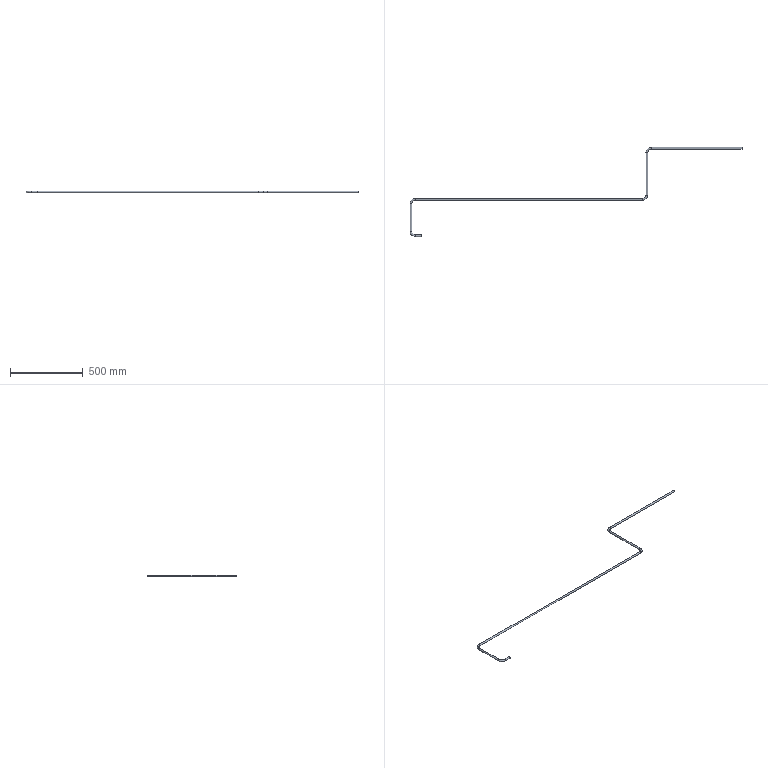Part | NX | features solid 2 | 1 solid | 11 faces | box 2287 x 613.706 x 12 mm | volume 328684 mm3 | cylinder 5 | torus 4 | plane 2 | commonest cylinder face diameters 12 x5
STEP:
#1=CARTESIAN_POINT('',(830.,756.706,-484.));
#2=VERTEX_POINT('',#1);
#3=CARTESIAN_POINT('',(830.,756.706,-490.));
#4=DIRECTION('',(1.,0.,0.));
#5=DIRECTION('',(0.,0.,1.));
#6=AXIS2_PLACEMENT_3D('',#3,#4,#5);
#7=CIRCLE('',#6,6.);
#8=EDGE_CURVE('',#2,#2,#7,.T.);
#9=ORIENTED_EDGE('',*,*,#8,.T.);
#10=EDGE_LOOP('',(#9));
#11=FACE_BOUND('',#10,.T.);
#12=CARTESIAN_POINT('',(1456.,756.706,-484.));
#13=VERTEX_POINT('',#12);
#14=CARTESIAN_POINT('',(1456.,756.706,-490.));
#15=DIRECTION('',(1.,0.,0.));
#16=DIRECTION('',(0.,0.,1.));
#17=AXIS2_PLACEMENT_3D('',#14,#15,#16);
#18=CIRCLE('',#17,6.);
#19=EDGE_CURVE('',#13,#13,#18,.T.);
#20=ORIENTED_EDGE('',*,*,#19,.F.);
#21=EDGE_LOOP('',(#20));
#22=FACE_BOUND('',#21,.T.);
#23=CARTESIAN_POINT('',(830.,756.706,-490.));
#24=DIRECTION('',(1.,0.,0.));
#25=DIRECTION('',(0.,1.,0.));
#26=AXIS2_PLACEMENT_3D('',#23,#24,#25);
#27=CYLINDRICAL_SURFACE('',#26,6.);
#28=ADVANCED_FACE('',(#11,#22),#27,.T.);
#29=CARTESIAN_POINT('',(800.,726.706,-484.));
#30=VERTEX_POINT('',#29);
#31=CARTESIAN_POINT('',(800.,726.706,-490.));
#32=DIRECTION('',(0.,1.,0.));
#33=DIRECTION('',(0.,0.,1.));
#34=AXIS2_PLACEMENT_3D('',#31,#32,#33);
#35=CIRCLE('',#34,6.);
#36=EDGE_CURVE('',#30,#30,#35,.T.);
#37=ORIENTED_EDGE('',*,*,#36,.T.);
#38=EDGE_LOOP('',(#37));
#39=FACE_BOUND('',#38,.T.);
#40=ORIENTED_EDGE('',*,*,#8,.F.);
#41=EDGE_LOOP('',(#40));
#42=FACE_BOUND('',#41,.T.);
#43=CARTESIAN_POINT('',(830.,726.706,-490.));
#44=DIRECTION('',(0.,0.,-1.));
#45=DIRECTION('',(-1.,0.,0.));
#46=AXIS2_PLACEMENT_3D('',#43,#44,#45);
#47=TOROIDAL_SURFACE('',#46,30.,6.);
#48=ADVANCED_FACE('',(#39,#42),#47,.T.);
#49=CARTESIAN_POINT('',(800.,435.,-484.));
#50=VERTEX_POINT('',#49);
#51=CARTESIAN_POINT('',(800.,435.,-490.));
#52=DIRECTION('',(0.,1.,0.));
#53=DIRECTION('',(0.,0.,1.));
#54=AXIS2_PLACEMENT_3D('',#51,#52,#53);
#55=CIRCLE('',#54,6.);
#56=EDGE_CURVE('',#50,#50,#55,.T.);
#57=ORIENTED_EDGE('',*,*,#56,.T.);
#58=EDGE_LOOP('',(#57));
#59=FACE_BOUND('',#58,.T.);
#60=ORIENTED_EDGE('',*,*,#36,.F.);
#61=EDGE_LOOP('',(#60));
#62=FACE_BOUND('',#61,.T.);
#63=CARTESIAN_POINT('',(800.,435.,-490.));
#64=DIRECTION('',(0.,1.,0.));
#65=DIRECTION('',(0.,0.,1.));
#66=AXIS2_PLACEMENT_3D('',#63,#64,#65);
#67=CYLINDRICAL_SURFACE('',#66,6.);
#68=ADVANCED_FACE('',(#59,#62),#67,.T.);
#69=CARTESIAN_POINT('',(770.,405.,-484.));
#70=VERTEX_POINT('',#69);
#71=CARTESIAN_POINT('',(770.,405.,-490.));
#72=DIRECTION('',(1.,0.,0.));
#73=DIRECTION('',(0.,0.,1.));
#74=AXIS2_PLACEMENT_3D('',#71,#72,#73);
#75=CIRCLE('',#74,6.);
#76=EDGE_CURVE('',#70,#70,#75,.T.);
#77=ORIENTED_EDGE('',*,*,#76,.T.);
#78=EDGE_LOOP('',(#77));
#79=FACE_BOUND('',#78,.T.);
#80=ORIENTED_EDGE('',*,*,#56,.F.);
#81=EDGE_LOOP('',(#80));
#82=FACE_BOUND('',#81,.T.);
#83=CARTESIAN_POINT('',(770.,435.,-490.));
#84=DIRECTION('',(0.,0.,1.));
#85=DIRECTION('',(1.,0.,0.));
#86=AXIS2_PLACEMENT_3D('',#83,#84,#85);
#87=TOROIDAL_SURFACE('',#86,30.,6.);
#88=ADVANCED_FACE('',(#79,#82),#87,.T.);
#89=CARTESIAN_POINT('',(-795.,405.,-484.));
#90=VERTEX_POINT('',#89);
#91=CARTESIAN_POINT('',(-795.,405.,-490.));
#92=DIRECTION('',(1.,0.,0.));
#93=DIRECTION('',(0.,0.,1.));
#94=AXIS2_PLACEMENT_3D('',#91,#92,#93);
#95=CIRCLE('',#94,6.);
#96=EDGE_CURVE('',#90,#90,#95,.T.);
#97=ORIENTED_EDGE('',*,*,#96,.T.);
#98=EDGE_LOOP('',(#97));
#99=FACE_BOUND('',#98,.T.);
#100=ORIENTED_EDGE('',*,*,#76,.F.);
#101=EDGE_LOOP('',(#100));
#102=FACE_BOUND('',#101,.T.);
#103=CARTESIAN_POINT('',(-795.,405.,-490.));
#104=DIRECTION('',(1.,0.,0.));
#105=DIRECTION('',(0.,0.,-1.));
#106=AXIS2_PLACEMENT_3D('',#103,#104,#105);
#107=CYLINDRICAL_SURFACE('',#106,6.);
#108=ADVANCED_FACE('',(#99,#102),#107,.T.);
#109=CARTESIAN_POINT('',(-825.,375.,-484.));
#110=VERTEX_POINT('',#109);
#111=CARTESIAN_POINT('',(-825.,375.,-490.));
#112=DIRECTION('',(0.,1.,0.));
#113=DIRECTION('',(0.,0.,1.));
#114=AXIS2_PLACEMENT_3D('',#111,#112,#113);
#115=CIRCLE('',#114,6.);
#116=EDGE_CURVE('',#110,#110,#115,.T.);
#117=ORIENTED_EDGE('',*,*,#116,.T.);
#118=EDGE_LOOP('',(#117));
#119=FACE_BOUND('',#118,.T.);
#120=ORIENTED_EDGE('',*,*,#96,.F.);
#121=EDGE_LOOP('',(#120));
#122=FACE_BOUND('',#121,.T.);
#123=CARTESIAN_POINT('',(-795.,375.,-490.));
#124=DIRECTION('',(0.,0.,-1.));
#125=DIRECTION('',(-1.,0.,0.));
#126=AXIS2_PLACEMENT_3D('',#123,#124,#125);
#127=TOROIDAL_SURFACE('',#126,30.,6.);
#128=ADVANCED_FACE('',(#119,#122),#127,.T.);
#129=CARTESIAN_POINT('',(-825.,185.,-484.));
#130=VERTEX_POINT('',#129);
#131=CARTESIAN_POINT('',(-825.,185.,-490.));
#132=DIRECTION('',(0.,1.,0.));
#133=DIRECTION('',(0.,0.,1.));
#134=AXIS2_PLACEMENT_3D('',#131,#132,#133);
#135=CIRCLE('',#134,6.);
#136=EDGE_CURVE('',#130,#130,#135,.T.);
#137=ORIENTED_EDGE('',*,*,#136,.T.);
#138=EDGE_LOOP('',(#137));
#139=FACE_BOUND('',#138,.T.);
#140=ORIENTED_EDGE('',*,*,#116,.F.);
#141=EDGE_LOOP('',(#140));
#142=FACE_BOUND('',#141,.T.);
#143=CARTESIAN_POINT('',(-825.,185.,-490.));
#144=DIRECTION('',(0.,1.,0.));
#145=DIRECTION('',(0.,0.,1.));
#146=AXIS2_PLACEMENT_3D('',#143,#144,#145);
#147=CYLINDRICAL_SURFACE('',#146,6.);
#148=ADVANCED_FACE('',(#139,#142),#147,.T.);
#149=CARTESIAN_POINT('',(-795.,155.,-484.));
#150=VERTEX_POINT('',#149);
#151=CARTESIAN_POINT('',(-795.,155.,-490.));
#152=DIRECTION('',(-1.,0.,0.));
#153=DIRECTION('',(0.,0.,1.));
#154=AXIS2_PLACEMENT_3D('',#151,#152,#153);
#155=CIRCLE('',#154,6.);
#156=EDGE_CURVE('',#150,#150,#155,.T.);
#157=ORIENTED_EDGE('',*,*,#156,.T.);
#158=EDGE_LOOP('',(#157));
#159=FACE_BOUND('',#158,.T.);
#160=ORIENTED_EDGE('',*,*,#136,.F.);
#161=EDGE_LOOP('',(#160));
#162=FACE_BOUND('',#161,.T.);
#163=CARTESIAN_POINT('',(-795.,185.,-490.));
#164=DIRECTION('',(0.,0.,-1.));
#165=DIRECTION('',(-1.,0.,0.));
#166=AXIS2_PLACEMENT_3D('',#163,#164,#165);
#167=TOROIDAL_SURFACE('',#166,30.,6.);
#168=ADVANCED_FACE('',(#159,#162),#167,.T.);
#169=ORIENTED_EDGE('',*,*,#156,.F.);
#170=EDGE_LOOP('',(#169));
#171=FACE_BOUND('',#170,.T.);
#172=CARTESIAN_POINT('',(-750.,155.,-484.));
#173=VERTEX_POINT('',#172);
#174=CARTESIAN_POINT('',(-750.,155.,-490.));
#175=DIRECTION('',(-1.,0.,0.));
#176=DIRECTION('',(0.,0.,1.));
#177=AXIS2_PLACEMENT_3D('',#174,#175,#176);
#178=CIRCLE('',#177,6.);
#179=EDGE_CURVE('',#173,#173,#178,.T.);
#180=ORIENTED_EDGE('',*,*,#179,.T.);
#181=EDGE_LOOP('',(#180));
#182=FACE_BOUND('',#181,.T.);
#183=CARTESIAN_POINT('',(-795.,155.,-490.));
#184=DIRECTION('',(1.,0.,0.));
#185=DIRECTION('',(0.,0.,-1.));
#186=AXIS2_PLACEMENT_3D('',#183,#184,#185);
#187=CYLINDRICAL_SURFACE('',#186,6.);
#188=ADVANCED_FACE('',(#171,#182),#187,.T.);
#189=ORIENTED_EDGE('',*,*,#19,.T.);
#190=EDGE_LOOP('',(#189));
#191=FACE_BOUND('',#190,.T.);
#192=CARTESIAN_POINT('',(1456.,756.706,-490.));
#193=DIRECTION('',(1.,0.,0.));
#194=DIRECTION('',(0.,0.,1.));
#195=AXIS2_PLACEMENT_3D('',#192,#193,#194);
#196=PLANE('',#195);
#197=ADVANCED_FACE('',(#191),#196,.T.);
#198=ORIENTED_EDGE('',*,*,#179,.F.);
#199=EDGE_LOOP('',(#198));
#200=FACE_BOUND('',#199,.T.);
#201=CARTESIAN_POINT('',(-750.,155.,-490.));
#202=DIRECTION('',(-1.,0.,0.));
#203=DIRECTION('',(0.,0.,1.));
#204=AXIS2_PLACEMENT_3D('',#201,#202,#203);
#205=PLANE('',#204);
#206=ADVANCED_FACE('',(#200),#205,.F.);
#207=CLOSED_SHELL('',(#28,#48,#68,#88,#108,#128,#148,#168,#188,#197,#206));
#208=MANIFOLD_SOLID_BREP('',#207);
#209=(LENGTH_UNIT()NAMED_UNIT(*)SI_UNIT(.MILLI.,.METRE.));
#210=UNCERTAINTY_MEASURE_WITH_UNIT(LENGTH_MEASURE(0.00001),#209,'','');
#211=(NAMED_UNIT(*)PLANE_ANGLE_UNIT()SI_UNIT($,.RADIAN.));
#212=(NAMED_UNIT(*)SI_UNIT($,.STERADIAN.)SOLID_ANGLE_UNIT());
#213=(GEOMETRIC_REPRESENTATION_CONTEXT(3)GLOBAL_UNCERTAINTY_ASSIGNED_CONTEXT((#210))GLOBAL_UNIT_ASSIGNED_CONTEXT((#209,#211,#212))REPRESENTATION_CONTEXT('',''));
#214=ADVANCED_BREP_SHAPE_REPRESENTATION('',(#208),#213);